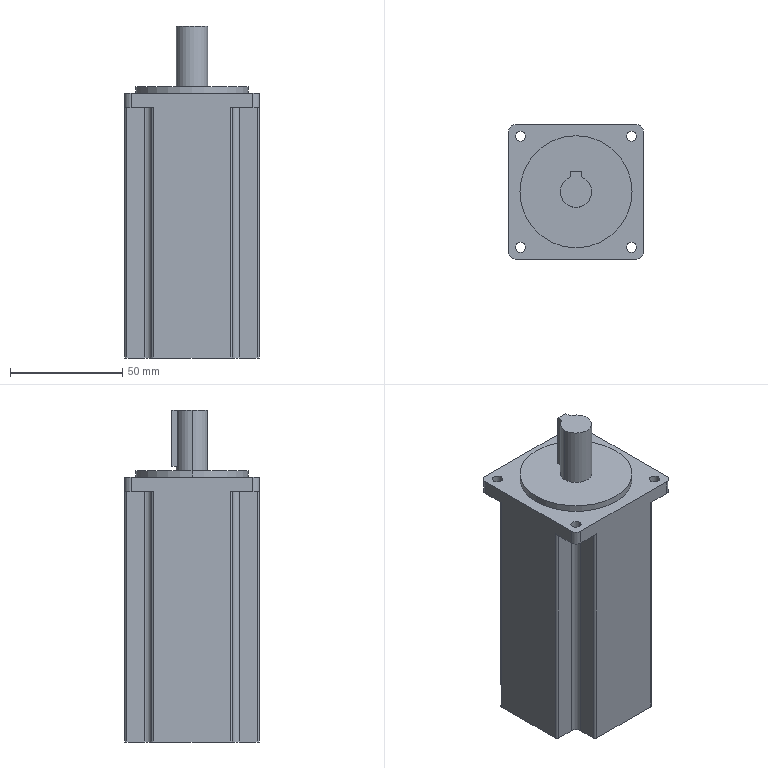Part | SolidWorks | features BaseBody 1 | 1 solid | 52 faces | box 60 x 60 x 148 mm | volume 371098 mm3 | cylinder 28 | plane 24 | commonest cylinder face diameters 2 x8 4.5 x8 6 x8 14 x2 50 x2